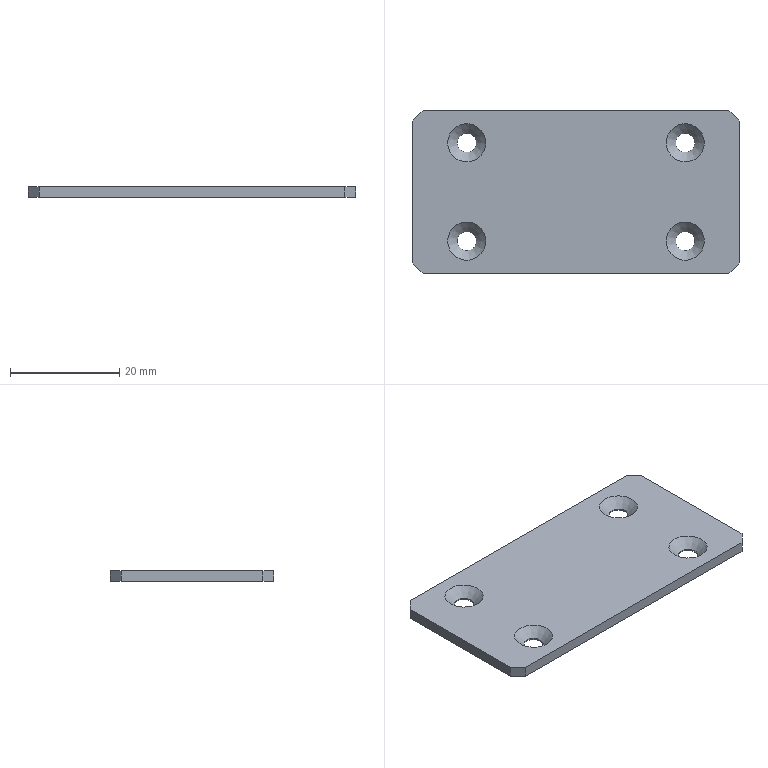Part | NX | 1 solid | 18 faces | box 60 x 30 x 2 mm | volume 3417 mm3 | plane 10 | cylinder 4 | cone 4 | commonest cylinder face diameters 3.5 x4
STEP:
#1=CARTESIAN_POINT('',(30.,-13.,2.));
#2=VERTEX_POINT('',#1);
#3=CARTESIAN_POINT('',(30.,13.,2.));
#4=VERTEX_POINT('',#3);
#5=CARTESIAN_POINT('',(30.,15.,2.));
#6=DIRECTION('',(0.,1.,0.));
#7=VECTOR('',#6,1000.);
#8=LINE('',#5,#7);
#9=EDGE_CURVE('',#2,#4,#8,.T.);
#10=ORIENTED_EDGE('',*,*,#9,.F.);
#11=CARTESIAN_POINT('',(30.,-13.,0.));
#12=VERTEX_POINT('',#11);
#13=CARTESIAN_POINT('',(30.,-13.,2.));
#14=DIRECTION('',(0.,0.,-1.));
#15=VECTOR('',#14,1000.);
#16=LINE('',#13,#15);
#17=EDGE_CURVE('',#2,#12,#16,.T.);
#18=ORIENTED_EDGE('',*,*,#17,.T.);
#19=CARTESIAN_POINT('',(30.,13.,0.));
#20=VERTEX_POINT('',#19);
#21=CARTESIAN_POINT('',(30.,15.,0.));
#22=DIRECTION('',(0.,1.,0.));
#23=VECTOR('',#22,1000.);
#24=LINE('',#21,#23);
#25=EDGE_CURVE('',#12,#20,#24,.T.);
#26=ORIENTED_EDGE('',*,*,#25,.T.);
#27=CARTESIAN_POINT('',(30.,13.,2.));
#28=DIRECTION('',(0.,0.,1.));
#29=VECTOR('',#28,1000.);
#30=LINE('',#27,#29);
#31=EDGE_CURVE('',#20,#4,#30,.T.);
#32=ORIENTED_EDGE('',*,*,#31,.T.);
#33=EDGE_LOOP('',(#10,#18,#26,#32));
#34=FACE_BOUND('',#33,.T.);
#35=CARTESIAN_POINT('',(30.,15.,2.));
#36=DIRECTION('',(-1.,0.,0.));
#37=DIRECTION('',(0.,-1.,0.));
#38=AXIS2_PLACEMENT_3D('',#35,#36,#37);
#39=PLANE('',#38);
#40=ADVANCED_FACE('',(#34),#39,.F.);
#41=CARTESIAN_POINT('',(28.,15.,2.));
#42=VERTEX_POINT('',#41);
#43=CARTESIAN_POINT('',(-28.,15.,2.));
#44=VERTEX_POINT('',#43);
#45=CARTESIAN_POINT('',(-30.,15.,2.));
#46=DIRECTION('',(-1.,0.,0.));
#47=VECTOR('',#46,1000.);
#48=LINE('',#45,#47);
#49=EDGE_CURVE('',#42,#44,#48,.T.);
#50=ORIENTED_EDGE('',*,*,#49,.F.);
#51=CARTESIAN_POINT('',(28.,15.,0.));
#52=VERTEX_POINT('',#51);
#53=CARTESIAN_POINT('',(28.,15.,2.));
#54=DIRECTION('',(0.,0.,-1.));
#55=VECTOR('',#54,1000.);
#56=LINE('',#53,#55);
#57=EDGE_CURVE('',#42,#52,#56,.T.);
#58=ORIENTED_EDGE('',*,*,#57,.T.);
#59=CARTESIAN_POINT('',(-28.,15.,0.));
#60=VERTEX_POINT('',#59);
#61=CARTESIAN_POINT('',(-30.,15.,0.));
#62=DIRECTION('',(-1.,0.,0.));
#63=VECTOR('',#62,1000.);
#64=LINE('',#61,#63);
#65=EDGE_CURVE('',#52,#60,#64,.T.);
#66=ORIENTED_EDGE('',*,*,#65,.T.);
#67=CARTESIAN_POINT('',(-28.,15.,2.));
#68=DIRECTION('',(0.,0.,1.));
#69=VECTOR('',#68,1000.);
#70=LINE('',#67,#69);
#71=EDGE_CURVE('',#60,#44,#70,.T.);
#72=ORIENTED_EDGE('',*,*,#71,.T.);
#73=EDGE_LOOP('',(#50,#58,#66,#72));
#74=FACE_BOUND('',#73,.T.);
#75=CARTESIAN_POINT('',(-30.,15.,2.));
#76=DIRECTION('',(0.,-1.,0.));
#77=DIRECTION('',(0.,0.,-1.));
#78=AXIS2_PLACEMENT_3D('',#75,#76,#77);
#79=PLANE('',#78);
#80=ADVANCED_FACE('',(#74),#79,.F.);
#81=CARTESIAN_POINT('',(-30.,13.,0.));
#82=VERTEX_POINT('',#81);
#83=CARTESIAN_POINT('',(-30.,-13.,0.));
#84=VERTEX_POINT('',#83);
#85=CARTESIAN_POINT('',(-30.,15.,0.));
#86=DIRECTION('',(0.,-1.,0.));
#87=VECTOR('',#86,1000.);
#88=LINE('',#85,#87);
#89=EDGE_CURVE('',#82,#84,#88,.T.);
#90=ORIENTED_EDGE('',*,*,#89,.T.);
#91=CARTESIAN_POINT('',(-30.,-13.,2.));
#92=VERTEX_POINT('',#91);
#93=CARTESIAN_POINT('',(-30.,-13.,2.));
#94=DIRECTION('',(0.,0.,1.));
#95=VECTOR('',#94,1000.);
#96=LINE('',#93,#95);
#97=EDGE_CURVE('',#84,#92,#96,.T.);
#98=ORIENTED_EDGE('',*,*,#97,.T.);
#99=CARTESIAN_POINT('',(-30.,13.,2.));
#100=VERTEX_POINT('',#99);
#101=CARTESIAN_POINT('',(-30.,15.,2.));
#102=DIRECTION('',(0.,-1.,0.));
#103=VECTOR('',#102,1000.);
#104=LINE('',#101,#103);
#105=EDGE_CURVE('',#100,#92,#104,.T.);
#106=ORIENTED_EDGE('',*,*,#105,.F.);
#107=CARTESIAN_POINT('',(-30.,13.,2.));
#108=DIRECTION('',(0.,0.,-1.));
#109=VECTOR('',#108,1000.);
#110=LINE('',#107,#109);
#111=EDGE_CURVE('',#100,#82,#110,.T.);
#112=ORIENTED_EDGE('',*,*,#111,.T.);
#113=EDGE_LOOP('',(#90,#98,#106,#112));
#114=FACE_BOUND('',#113,.T.);
#115=CARTESIAN_POINT('',(-30.,15.,2.));
#116=DIRECTION('',(1.,0.,0.));
#117=DIRECTION('',(0.,1.,0.));
#118=AXIS2_PLACEMENT_3D('',#115,#116,#117);
#119=PLANE('',#118);
#120=ADVANCED_FACE('',(#114),#119,.F.);
#121=CARTESIAN_POINT('',(-28.,-15.,0.));
#122=VERTEX_POINT('',#121);
#123=CARTESIAN_POINT('',(28.,-15.,0.));
#124=VERTEX_POINT('',#123);
#125=CARTESIAN_POINT('',(-30.,-15.,0.));
#126=DIRECTION('',(1.,0.,0.));
#127=VECTOR('',#126,1000.);
#128=LINE('',#125,#127);
#129=EDGE_CURVE('',#122,#124,#128,.T.);
#130=ORIENTED_EDGE('',*,*,#129,.T.);
#131=CARTESIAN_POINT('',(28.,-15.,2.));
#132=VERTEX_POINT('',#131);
#133=CARTESIAN_POINT('',(28.,-15.,2.));
#134=DIRECTION('',(0.,0.,1.));
#135=VECTOR('',#134,1000.);
#136=LINE('',#133,#135);
#137=EDGE_CURVE('',#124,#132,#136,.T.);
#138=ORIENTED_EDGE('',*,*,#137,.T.);
#139=CARTESIAN_POINT('',(-28.,-15.,2.));
#140=VERTEX_POINT('',#139);
#141=CARTESIAN_POINT('',(-30.,-15.,2.));
#142=DIRECTION('',(1.,0.,0.));
#143=VECTOR('',#142,1000.);
#144=LINE('',#141,#143);
#145=EDGE_CURVE('',#140,#132,#144,.T.);
#146=ORIENTED_EDGE('',*,*,#145,.F.);
#147=CARTESIAN_POINT('',(-28.,-15.,2.));
#148=DIRECTION('',(0.,0.,-1.));
#149=VECTOR('',#148,1000.);
#150=LINE('',#147,#149);
#151=EDGE_CURVE('',#140,#122,#150,.T.);
#152=ORIENTED_EDGE('',*,*,#151,.T.);
#153=EDGE_LOOP('',(#130,#138,#146,#152));
#154=FACE_BOUND('',#153,.T.);
#155=CARTESIAN_POINT('',(-30.,-15.,2.));
#156=DIRECTION('',(0.,1.,0.));
#157=DIRECTION('',(0.,0.,1.));
#158=AXIS2_PLACEMENT_3D('',#155,#156,#157);
#159=PLANE('',#158);
#160=ADVANCED_FACE('',(#154),#159,.F.);
#161=CARTESIAN_POINT('',(-16.5,-9.,2.));
#162=VERTEX_POINT('',#161);
#163=CARTESIAN_POINT('',(-20.,-9.,2.));
#164=DIRECTION('',(0.,0.,1.));
#165=DIRECTION('',(1.,0.,0.));
#166=AXIS2_PLACEMENT_3D('',#163,#164,#165);
#167=CIRCLE('',#166,3.5);
#168=EDGE_CURVE('',#162,#162,#167,.T.);
#169=ORIENTED_EDGE('',*,*,#168,.F.);
#170=EDGE_LOOP('',(#169));
#171=FACE_BOUND('',#170,.T.);
#172=CARTESIAN_POINT('',(23.5,9.,2.));
#173=VERTEX_POINT('',#172);
#174=CARTESIAN_POINT('',(20.,9.,2.));
#175=DIRECTION('',(0.,0.,1.));
#176=DIRECTION('',(1.,0.,0.));
#177=AXIS2_PLACEMENT_3D('',#174,#175,#176);
#178=CIRCLE('',#177,3.5);
#179=EDGE_CURVE('',#173,#173,#178,.T.);
#180=ORIENTED_EDGE('',*,*,#179,.F.);
#181=EDGE_LOOP('',(#180));
#182=FACE_BOUND('',#181,.T.);
#183=CARTESIAN_POINT('',(23.5,-9.,2.));
#184=VERTEX_POINT('',#183);
#185=CARTESIAN_POINT('',(20.,-9.,2.));
#186=DIRECTION('',(0.,0.,1.));
#187=DIRECTION('',(1.,0.,0.));
#188=AXIS2_PLACEMENT_3D('',#185,#186,#187);
#189=CIRCLE('',#188,3.5);
#190=EDGE_CURVE('',#184,#184,#189,.T.);
#191=ORIENTED_EDGE('',*,*,#190,.F.);
#192=EDGE_LOOP('',(#191));
#193=FACE_BOUND('',#192,.T.);
#194=CARTESIAN_POINT('',(-16.5,9.,2.));
#195=VERTEX_POINT('',#194);
#196=CARTESIAN_POINT('',(-20.,9.,2.));
#197=DIRECTION('',(0.,0.,1.));
#198=DIRECTION('',(1.,0.,0.));
#199=AXIS2_PLACEMENT_3D('',#196,#197,#198);
#200=CIRCLE('',#199,3.5);
#201=EDGE_CURVE('',#195,#195,#200,.T.);
#202=ORIENTED_EDGE('',*,*,#201,.F.);
#203=EDGE_LOOP('',(#202));
#204=FACE_BOUND('',#203,.T.);
#205=ORIENTED_EDGE('',*,*,#145,.T.);
#206=CARTESIAN_POINT('',(21.5,-21.5,2.));
#207=DIRECTION('',(-0.7071,-0.7071,0.));
#208=VECTOR('',#207,1000.);
#209=LINE('',#206,#208);
#210=EDGE_CURVE('',#132,#2,#209,.F.);
#211=ORIENTED_EDGE('',*,*,#210,.T.);
#212=ORIENTED_EDGE('',*,*,#9,.T.);
#213=CARTESIAN_POINT('',(21.5,21.5,2.));
#214=DIRECTION('',(0.7071,-0.7071,0.));
#215=VECTOR('',#214,1000.);
#216=LINE('',#213,#215);
#217=EDGE_CURVE('',#4,#42,#216,.F.);
#218=ORIENTED_EDGE('',*,*,#217,.T.);
#219=ORIENTED_EDGE('',*,*,#49,.T.);
#220=CARTESIAN_POINT('',(-21.5,21.5,2.));
#221=DIRECTION('',(0.7071,0.7071,0.));
#222=VECTOR('',#221,1000.);
#223=LINE('',#220,#222);
#224=EDGE_CURVE('',#44,#100,#223,.F.);
#225=ORIENTED_EDGE('',*,*,#224,.T.);
#226=ORIENTED_EDGE('',*,*,#105,.T.);
#227=CARTESIAN_POINT('',(-21.5,-21.5,2.));
#228=DIRECTION('',(-0.7071,0.7071,0.));
#229=VECTOR('',#228,1000.);
#230=LINE('',#227,#229);
#231=EDGE_CURVE('',#92,#140,#230,.F.);
#232=ORIENTED_EDGE('',*,*,#231,.T.);
#233=EDGE_LOOP('',(#205,#211,#212,#218,#219,#225,#226,#232));
#234=FACE_BOUND('',#233,.T.);
#235=CARTESIAN_POINT('',(0.,0.,2.));
#236=DIRECTION('',(0.,0.,1.));
#237=DIRECTION('',(1.,0.,0.));
#238=AXIS2_PLACEMENT_3D('',#235,#236,#237);
#239=PLANE('',#238);
#240=ADVANCED_FACE('',(#171,#182,#193,#204,#234),#239,.T.);
#241=CARTESIAN_POINT('',(-18.25,-9.,0.));
#242=VERTEX_POINT('',#241);
#243=CARTESIAN_POINT('',(-20.,-9.,0.));
#244=DIRECTION('',(0.,0.,1.));
#245=DIRECTION('',(1.,0.,0.));
#246=AXIS2_PLACEMENT_3D('',#243,#244,#245);
#247=CIRCLE('',#246,1.75);
#248=EDGE_CURVE('',#242,#242,#247,.T.);
#249=ORIENTED_EDGE('',*,*,#248,.T.);
#250=EDGE_LOOP('',(#249));
#251=FACE_BOUND('',#250,.T.);
#252=CARTESIAN_POINT('',(21.75,9.,0.));
#253=VERTEX_POINT('',#252);
#254=CARTESIAN_POINT('',(20.,9.,0.));
#255=DIRECTION('',(0.,0.,1.));
#256=DIRECTION('',(1.,0.,0.));
#257=AXIS2_PLACEMENT_3D('',#254,#255,#256);
#258=CIRCLE('',#257,1.75);
#259=EDGE_CURVE('',#253,#253,#258,.T.);
#260=ORIENTED_EDGE('',*,*,#259,.T.);
#261=EDGE_LOOP('',(#260));
#262=FACE_BOUND('',#261,.T.);
#263=CARTESIAN_POINT('',(21.75,-9.,0.));
#264=VERTEX_POINT('',#263);
#265=CARTESIAN_POINT('',(20.,-9.,0.));
#266=DIRECTION('',(0.,0.,1.));
#267=DIRECTION('',(1.,0.,0.));
#268=AXIS2_PLACEMENT_3D('',#265,#266,#267);
#269=CIRCLE('',#268,1.75);
#270=EDGE_CURVE('',#264,#264,#269,.T.);
#271=ORIENTED_EDGE('',*,*,#270,.T.);
#272=EDGE_LOOP('',(#271));
#273=FACE_BOUND('',#272,.T.);
#274=CARTESIAN_POINT('',(-18.25,9.,0.));
#275=VERTEX_POINT('',#274);
#276=CARTESIAN_POINT('',(-20.,9.,0.));
#277=DIRECTION('',(0.,0.,1.));
#278=DIRECTION('',(1.,0.,0.));
#279=AXIS2_PLACEMENT_3D('',#276,#277,#278);
#280=CIRCLE('',#279,1.75);
#281=EDGE_CURVE('',#275,#275,#280,.T.);
#282=ORIENTED_EDGE('',*,*,#281,.T.);
#283=EDGE_LOOP('',(#282));
#284=FACE_BOUND('',#283,.T.);
#285=ORIENTED_EDGE('',*,*,#25,.F.);
#286=CARTESIAN_POINT('',(30.,-13.,0.));
#287=DIRECTION('',(0.7071,0.7071,0.));
#288=VECTOR('',#287,1000.);
#289=LINE('',#286,#288);
#290=EDGE_CURVE('',#12,#124,#289,.F.);
#291=ORIENTED_EDGE('',*,*,#290,.T.);
#292=ORIENTED_EDGE('',*,*,#129,.F.);
#293=CARTESIAN_POINT('',(-28.,-15.,0.));
#294=DIRECTION('',(0.7071,-0.7071,0.));
#295=VECTOR('',#294,1000.);
#296=LINE('',#293,#295);
#297=EDGE_CURVE('',#122,#84,#296,.F.);
#298=ORIENTED_EDGE('',*,*,#297,.T.);
#299=ORIENTED_EDGE('',*,*,#89,.F.);
#300=CARTESIAN_POINT('',(-30.,13.,0.));
#301=DIRECTION('',(-0.7071,-0.7071,0.));
#302=VECTOR('',#301,1000.);
#303=LINE('',#300,#302);
#304=EDGE_CURVE('',#82,#60,#303,.F.);
#305=ORIENTED_EDGE('',*,*,#304,.T.);
#306=ORIENTED_EDGE('',*,*,#65,.F.);
#307=CARTESIAN_POINT('',(28.,15.,0.));
#308=DIRECTION('',(-0.7071,0.7071,0.));
#309=VECTOR('',#308,1000.);
#310=LINE('',#307,#309);
#311=EDGE_CURVE('',#52,#20,#310,.F.);
#312=ORIENTED_EDGE('',*,*,#311,.T.);
#313=EDGE_LOOP('',(#285,#291,#292,#298,#299,#305,#306,#312));
#314=FACE_BOUND('',#313,.T.);
#315=CARTESIAN_POINT('',(0.,0.,0.));
#316=DIRECTION('',(0.,0.,1.));
#317=DIRECTION('',(1.,0.,0.));
#318=AXIS2_PLACEMENT_3D('',#315,#316,#317);
#319=PLANE('',#318);
#320=ADVANCED_FACE('',(#251,#262,#273,#284,#314),#319,.F.);
#321=ORIENTED_EDGE('',*,*,#281,.F.);
#322=EDGE_LOOP('',(#321));
#323=FACE_BOUND('',#322,.T.);
#324=CARTESIAN_POINT('',(-18.25,9.,0.25));
#325=VERTEX_POINT('',#324);
#326=CARTESIAN_POINT('',(-20.,9.,0.25));
#327=DIRECTION('',(0.,0.,1.));
#328=DIRECTION('',(1.,0.,0.));
#329=AXIS2_PLACEMENT_3D('',#326,#327,#328);
#330=CIRCLE('',#329,1.75);
#331=EDGE_CURVE('',#325,#325,#330,.T.);
#332=ORIENTED_EDGE('',*,*,#331,.T.);
#333=EDGE_LOOP('',(#332));
#334=FACE_BOUND('',#333,.T.);
#335=CARTESIAN_POINT('',(-20.,9.,2.));
#336=DIRECTION('',(0.,0.,1.));
#337=DIRECTION('',(1.,0.,0.));
#338=AXIS2_PLACEMENT_3D('',#335,#336,#337);
#339=CYLINDRICAL_SURFACE('',#338,1.75);
#340=ADVANCED_FACE('',(#323,#334),#339,.F.);
#341=ORIENTED_EDGE('',*,*,#331,.F.);
#342=EDGE_LOOP('',(#341));
#343=FACE_BOUND('',#342,.T.);
#344=ORIENTED_EDGE('',*,*,#201,.T.);
#345=EDGE_LOOP('',(#344));
#346=FACE_BOUND('',#345,.T.);
#347=CARTESIAN_POINT('',(-20.,9.,2.));
#348=DIRECTION('',(0.,0.,1.));
#349=DIRECTION('',(1.,0.,0.));
#350=AXIS2_PLACEMENT_3D('',#347,#348,#349);
#351=CONICAL_SURFACE('',#350,3.5,0.7854);
#352=ADVANCED_FACE('',(#343,#346),#351,.F.);
#353=ORIENTED_EDGE('',*,*,#270,.F.);
#354=EDGE_LOOP('',(#353));
#355=FACE_BOUND('',#354,.T.);
#356=CARTESIAN_POINT('',(21.75,-9.,0.25));
#357=VERTEX_POINT('',#356);
#358=CARTESIAN_POINT('',(20.,-9.,0.25));
#359=DIRECTION('',(0.,0.,1.));
#360=DIRECTION('',(1.,0.,0.));
#361=AXIS2_PLACEMENT_3D('',#358,#359,#360);
#362=CIRCLE('',#361,1.75);
#363=EDGE_CURVE('',#357,#357,#362,.T.);
#364=ORIENTED_EDGE('',*,*,#363,.T.);
#365=EDGE_LOOP('',(#364));
#366=FACE_BOUND('',#365,.T.);
#367=CARTESIAN_POINT('',(20.,-9.,2.));
#368=DIRECTION('',(0.,0.,1.));
#369=DIRECTION('',(1.,0.,0.));
#370=AXIS2_PLACEMENT_3D('',#367,#368,#369);
#371=CYLINDRICAL_SURFACE('',#370,1.75);
#372=ADVANCED_FACE('',(#355,#366),#371,.F.);
#373=ORIENTED_EDGE('',*,*,#363,.F.);
#374=EDGE_LOOP('',(#373));
#375=FACE_BOUND('',#374,.T.);
#376=ORIENTED_EDGE('',*,*,#190,.T.);
#377=EDGE_LOOP('',(#376));
#378=FACE_BOUND('',#377,.T.);
#379=CARTESIAN_POINT('',(20.,-9.,2.));
#380=DIRECTION('',(0.,0.,1.));
#381=DIRECTION('',(1.,0.,0.));
#382=AXIS2_PLACEMENT_3D('',#379,#380,#381);
#383=CONICAL_SURFACE('',#382,3.5,0.7854);
#384=ADVANCED_FACE('',(#375,#378),#383,.F.);
#385=ORIENTED_EDGE('',*,*,#259,.F.);
#386=EDGE_LOOP('',(#385));
#387=FACE_BOUND('',#386,.T.);
#388=CARTESIAN_POINT('',(21.75,9.,0.25));
#389=VERTEX_POINT('',#388);
#390=CARTESIAN_POINT('',(20.,9.,0.25));
#391=DIRECTION('',(0.,0.,1.));
#392=DIRECTION('',(1.,0.,0.));
#393=AXIS2_PLACEMENT_3D('',#390,#391,#392);
#394=CIRCLE('',#393,1.75);
#395=EDGE_CURVE('',#389,#389,#394,.T.);
#396=ORIENTED_EDGE('',*,*,#395,.T.);
#397=EDGE_LOOP('',(#396));
#398=FACE_BOUND('',#397,.T.);
#399=CARTESIAN_POINT('',(20.,9.,2.));
#400=DIRECTION('',(0.,0.,1.));
#401=DIRECTION('',(1.,0.,0.));
#402=AXIS2_PLACEMENT_3D('',#399,#400,#401);
#403=CYLINDRICAL_SURFACE('',#402,1.75);
#404=ADVANCED_FACE('',(#387,#398),#403,.F.);
#405=ORIENTED_EDGE('',*,*,#395,.F.);
#406=EDGE_LOOP('',(#405));
#407=FACE_BOUND('',#406,.T.);
#408=ORIENTED_EDGE('',*,*,#179,.T.);
#409=EDGE_LOOP('',(#408));
#410=FACE_BOUND('',#409,.T.);
#411=CARTESIAN_POINT('',(20.,9.,2.));
#412=DIRECTION('',(0.,0.,1.));
#413=DIRECTION('',(1.,0.,0.));
#414=AXIS2_PLACEMENT_3D('',#411,#412,#413);
#415=CONICAL_SURFACE('',#414,3.5,0.7854);
#416=ADVANCED_FACE('',(#407,#410),#415,.F.);
#417=ORIENTED_EDGE('',*,*,#248,.F.);
#418=EDGE_LOOP('',(#417));
#419=FACE_BOUND('',#418,.T.);
#420=CARTESIAN_POINT('',(-18.25,-9.,0.25));
#421=VERTEX_POINT('',#420);
#422=CARTESIAN_POINT('',(-20.,-9.,0.25));
#423=DIRECTION('',(0.,0.,1.));
#424=DIRECTION('',(1.,0.,0.));
#425=AXIS2_PLACEMENT_3D('',#422,#423,#424);
#426=CIRCLE('',#425,1.75);
#427=EDGE_CURVE('',#421,#421,#426,.T.);
#428=ORIENTED_EDGE('',*,*,#427,.T.);
#429=EDGE_LOOP('',(#428));
#430=FACE_BOUND('',#429,.T.);
#431=CARTESIAN_POINT('',(-20.,-9.,2.));
#432=DIRECTION('',(0.,0.,1.));
#433=DIRECTION('',(1.,0.,0.));
#434=AXIS2_PLACEMENT_3D('',#431,#432,#433);
#435=CYLINDRICAL_SURFACE('',#434,1.75);
#436=ADVANCED_FACE('',(#419,#430),#435,.F.);
#437=ORIENTED_EDGE('',*,*,#427,.F.);
#438=EDGE_LOOP('',(#437));
#439=FACE_BOUND('',#438,.T.);
#440=ORIENTED_EDGE('',*,*,#168,.T.);
#441=EDGE_LOOP('',(#440));
#442=FACE_BOUND('',#441,.T.);
#443=CARTESIAN_POINT('',(-20.,-9.,2.));
#444=DIRECTION('',(0.,0.,1.));
#445=DIRECTION('',(1.,0.,0.));
#446=AXIS2_PLACEMENT_3D('',#443,#444,#445);
#447=CONICAL_SURFACE('',#446,3.5,0.7854);
#448=ADVANCED_FACE('',(#439,#442),#447,.F.);
#449=ORIENTED_EDGE('',*,*,#210,.F.);
#450=ORIENTED_EDGE('',*,*,#137,.F.);
#451=ORIENTED_EDGE('',*,*,#290,.F.);
#452=ORIENTED_EDGE('',*,*,#17,.F.);
#453=EDGE_LOOP('',(#449,#450,#451,#452));
#454=FACE_BOUND('',#453,.T.);
#455=CARTESIAN_POINT('',(30.,-13.,2.));
#456=DIRECTION('',(-0.7071,0.7071,0.));
#457=DIRECTION('',(0.,0.,-1.));
#458=AXIS2_PLACEMENT_3D('',#455,#456,#457);
#459=PLANE('',#458);
#460=ADVANCED_FACE('',(#454),#459,.F.);
#461=ORIENTED_EDGE('',*,*,#217,.F.);
#462=ORIENTED_EDGE('',*,*,#31,.F.);
#463=ORIENTED_EDGE('',*,*,#311,.F.);
#464=ORIENTED_EDGE('',*,*,#57,.F.);
#465=EDGE_LOOP('',(#461,#462,#463,#464));
#466=FACE_BOUND('',#465,.T.);
#467=CARTESIAN_POINT('',(28.,15.,2.));
#468=DIRECTION('',(-0.7071,-0.7071,0.));
#469=DIRECTION('',(0.,0.,-1.));
#470=AXIS2_PLACEMENT_3D('',#467,#468,#469);
#471=PLANE('',#470);
#472=ADVANCED_FACE('',(#466),#471,.F.);
#473=ORIENTED_EDGE('',*,*,#231,.F.);
#474=ORIENTED_EDGE('',*,*,#97,.F.);
#475=ORIENTED_EDGE('',*,*,#297,.F.);
#476=ORIENTED_EDGE('',*,*,#151,.F.);
#477=EDGE_LOOP('',(#473,#474,#475,#476));
#478=FACE_BOUND('',#477,.T.);
#479=CARTESIAN_POINT('',(-28.,-15.,2.));
#480=DIRECTION('',(0.7071,0.7071,0.));
#481=DIRECTION('',(0.,0.,-1.));
#482=AXIS2_PLACEMENT_3D('',#479,#480,#481);
#483=PLANE('',#482);
#484=ADVANCED_FACE('',(#478),#483,.F.);
#485=ORIENTED_EDGE('',*,*,#224,.F.);
#486=ORIENTED_EDGE('',*,*,#71,.F.);
#487=ORIENTED_EDGE('',*,*,#304,.F.);
#488=ORIENTED_EDGE('',*,*,#111,.F.);
#489=EDGE_LOOP('',(#485,#486,#487,#488));
#490=FACE_BOUND('',#489,.T.);
#491=CARTESIAN_POINT('',(-30.,13.,2.));
#492=DIRECTION('',(0.7071,-0.7071,0.));
#493=DIRECTION('',(0.,0.,-1.));
#494=AXIS2_PLACEMENT_3D('',#491,#492,#493);
#495=PLANE('',#494);
#496=ADVANCED_FACE('',(#490),#495,.F.);
#497=CLOSED_SHELL('',(#40,#80,#120,#160,#240,#320,#340,#352,#372,#384,#404,#416,#436,#448,#460,#472,#484,#496));
#498=MANIFOLD_SOLID_BREP('',#497);
#499=(LENGTH_UNIT()NAMED_UNIT(*)SI_UNIT(.MILLI.,.METRE.));
#500=UNCERTAINTY_MEASURE_WITH_UNIT(LENGTH_MEASURE(0.00001),#499,'','');
#501=(NAMED_UNIT(*)PLANE_ANGLE_UNIT()SI_UNIT($,.RADIAN.));
#502=(NAMED_UNIT(*)SI_UNIT($,.STERADIAN.)SOLID_ANGLE_UNIT());
#503=(GEOMETRIC_REPRESENTATION_CONTEXT(3)GLOBAL_UNCERTAINTY_ASSIGNED_CONTEXT((#500))GLOBAL_UNIT_ASSIGNED_CONTEXT((#499,#501,#502))REPRESENTATION_CONTEXT('',''));
#504=ADVANCED_BREP_SHAPE_REPRESENTATION('',(#498),#503);